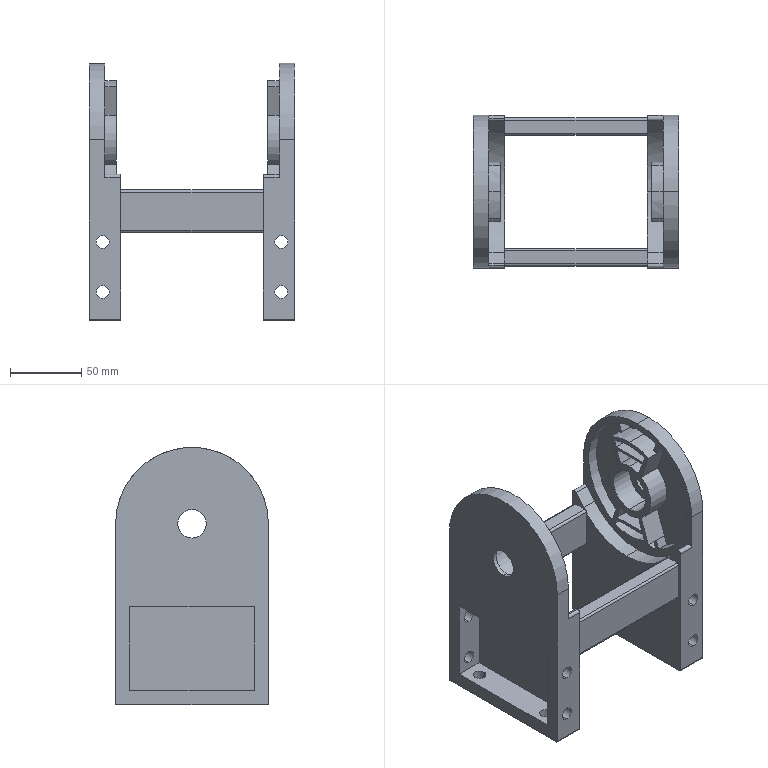Part | SolidWorks | features BaseBody 1 | 1 solid | 198 faces | box 144 x 107 x 180 mm | volume 373805 mm3 | plane 106 | cylinder 92 | commonest cylinder face diameters 9 x24 97 x11 41.6 x10 3 x8 4 x6 77 x6